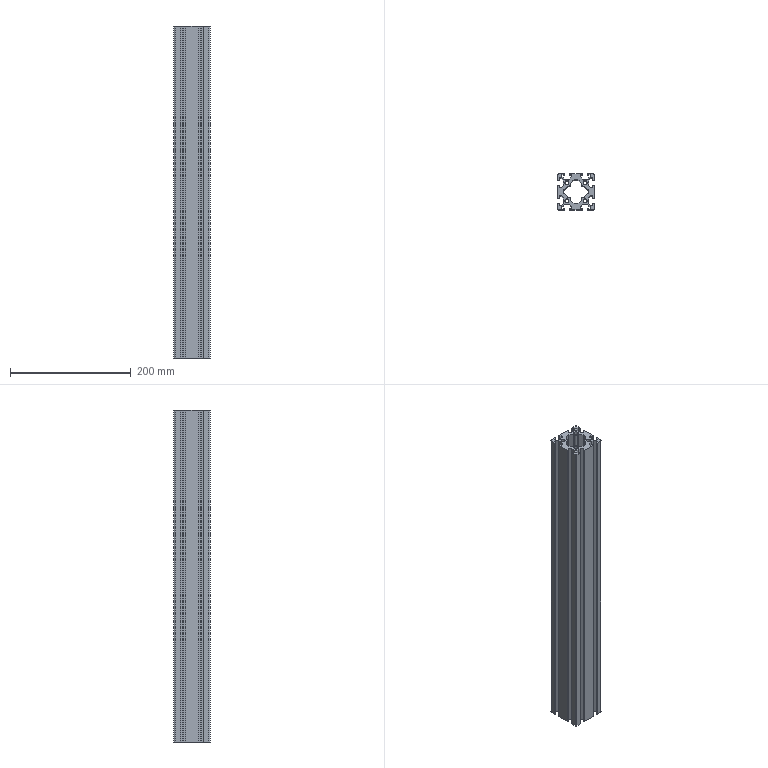Part | NX | features BREP 1 | 1 solid | 178 faces | box 60 x 60 x 550 mm | volume 841063 mm3 | plane 130 | cylinder 48 | commonest cylinder face diameters 0.6 x16 2 x16 6.8 x8 4 x4 6 x4